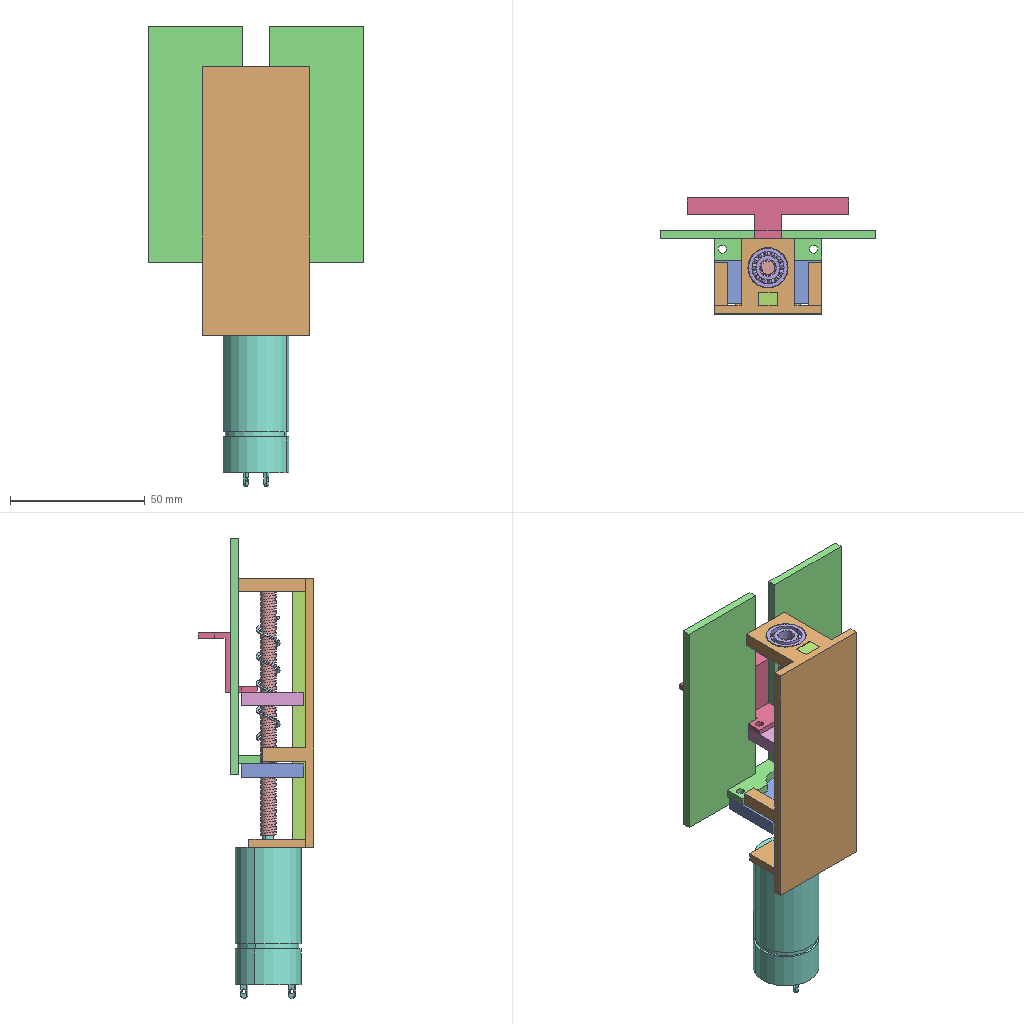Assembly | SolidWorks | 10 different items | 10 placed | box 80 x 43 x 171 mm
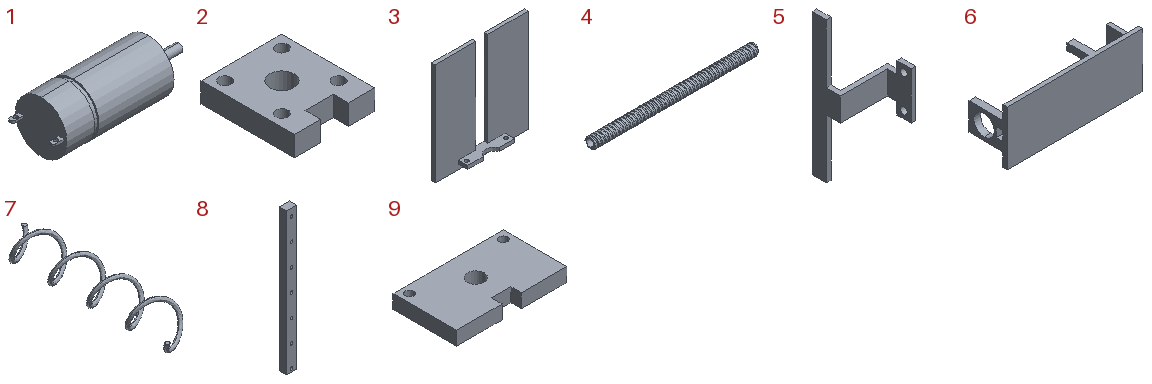Parts list (item | name | quantity | size | volume | features):
1 | - | x1 | 70.5 x 24.5 x 24.5 mm | 24091 mm3 | features ICE 4, Extrusion 1, Fillet 1, RevCut 1
2 | - | x1 | 20 x 23 x 5 mm | 1884 mm3 | features Extrusion 1
3 | - | x1 | 80 x 11 x 88 mm | 19474 mm3 | features Extrusion 1, ICE 1
4 | - | x1 | 92 x 6 x 6 mm | 2029 mm3 | features ICE 2, Cut 1, Helix 1, Revolution 1, SweepCut 1
5 | - | x1 | 22 x 22 x 60 mm | 1532 mm3 | features ICE 2, Extrusion 1
6 | - | x1 | 100 x 28 x 40 mm | 15612 mm3 | features ICE 5, Extrusion 1
7 | - | x1 | 9 x 46 x 9 mm | 88.855 mm3 | features Helix 1, Sweep 1
8 | - | x1 | 7 x 4.8 x 97 mm | 2868 mm3 | features ICE 2, Extrusion 1, LPattern 1
9 | - | x1 | 40 x 23 x 5 mm | 4255 mm3 | features Extrusion 1
10 | angular contact ball bearings gb | x1 | - | - | -
Mates (type | each side: item.copy, entity, surface, feature):
Coincident | 9.1 face plane Boss-Extrude1 | 8.1 face plane Boss-Extrude1 | 2 times
Concentric | 4.1 face cylinder Revolve1 | 2.1 face cylinder Boss-Extrude1
Coincident | 8.1 face plane Boss-Extrude1 | 2.1 face plane Boss-Extrude1
Coincident | 8.1 plane | assembly plane | 3 times
Concentric | 4.1 face cylinder Revolve1 | 1.1 face cylinder Boss-Extrude4
Coincident | 8.1 face plane Boss-Extrude1 | 6.1 face plane Boss-Extrude1
Coincident | 9.1 face plane Boss-Extrude1 | 3.1 face plane Boss-Extrude1
Concentric | 9.1 face cylinder Boss-Extrude1 | 3.1 face cylinder Boss-Extrude1 | 2 times
Coincident | 2.1 face plane Boss-Extrude1 | 5.1 face plane Boss-Extrude1
Concentric | 2.1 face cylinder Boss-Extrude1 | 5.1 face cylinder Boss-Extrude2 | 2 times
Coincident | 1.1 face plane Boss-Extrude1 | 6.1 face plane Boss-Extrude1
Coincident | 4.1 face plane Cut-Extrude1 | 1.1 face plane Boss-Extrude4
Coincident | 8.1 face plane Boss-Extrude1 | 6.1 face plane Boss-Extrude5
LimitDistanceDim | 6.1 face plane Boss-Extrude5 | 9.1 face plane Boss-Extrude1
LimitDistanceDim | 6.1 face plane Boss-Extrude5 | 2.1 face plane Boss-Extrude1
Coincident | 4.1 plane | 7.1 plane | 2 times
LimitDistanceDim | 3.1 face plane Boss-Extrude1 | 2.1 face plane Boss-Extrude1